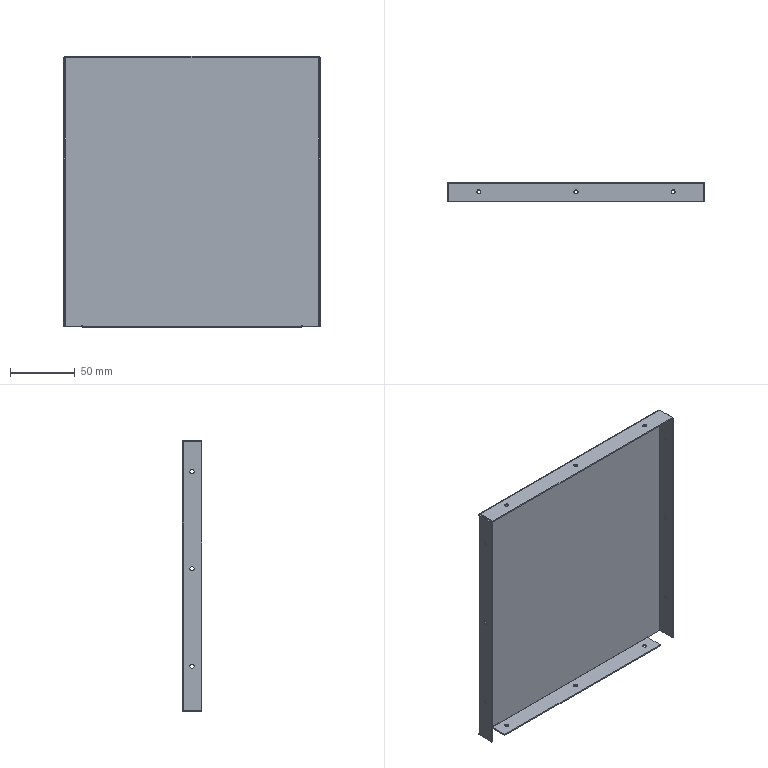Part | STEP file | TL42B-88D-2-plate heat exchanger 2 | 1 solid | 66 faces | box 198 x 15 x 209 mm | volume 51964 mm3 | plane 34 | cylinder 32 | commonest cylinder face diameters 3.2 x24 0.2 x4 2.2 x4